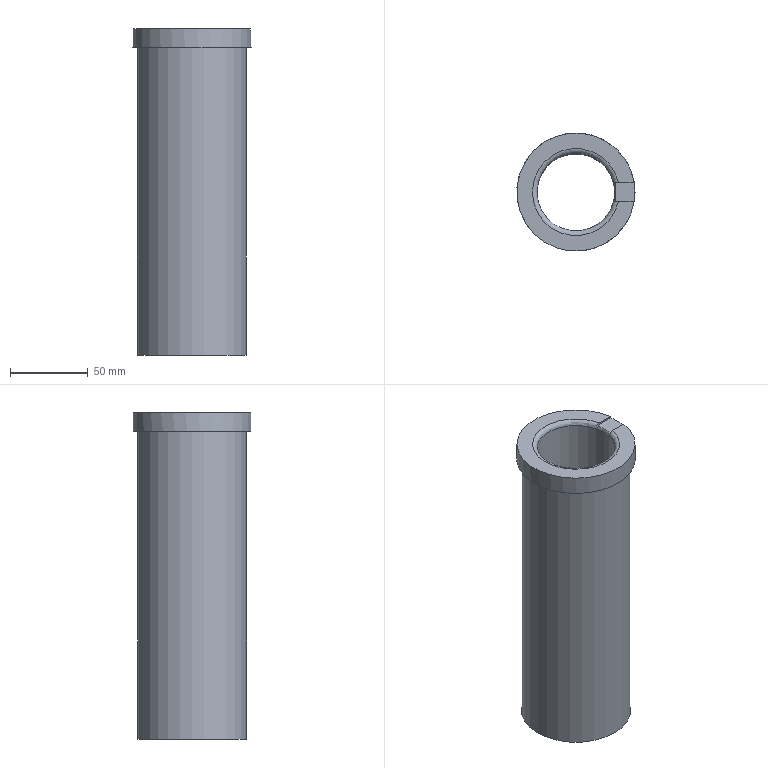Part | STEP file | solid 126 | 1 solid | 11 faces | box 76 x 76 x 210 mm | volume 403335 mm3 | plane 6 | cylinder 3 | torus 2 | commonest cylinder face diameters 50 x1 70 x1 76 x1